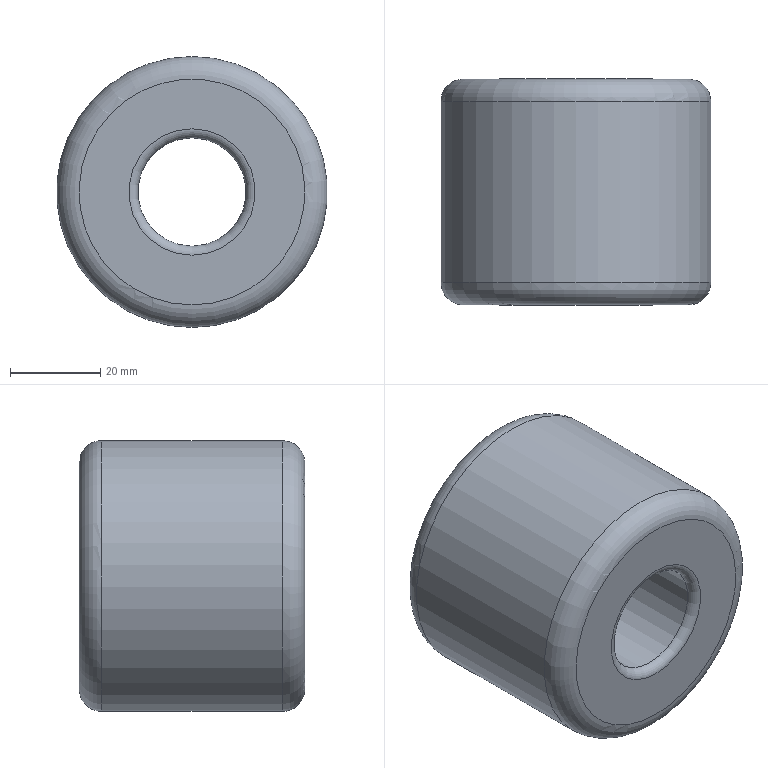Part | NX | features solid 2 | 1 solid | 8 faces | box 60 x 50 x 60 mm | volume 116671 mm3 | torus 4 | cylinder 2 | plane 2 | commonest cylinder face diameters 24 x1 60 x1
STEP:
#1=CARTESIAN_POINT('',(460.,445.,-55.));
#2=VERTEX_POINT('',#1);
#3=CARTESIAN_POINT('',(460.,445.,-25.));
#4=DIRECTION('',(0.,-1.,0.));
#5=DIRECTION('',(0.,0.,-1.));
#6=AXIS2_PLACEMENT_3D('',#3,#4,#5);
#7=CIRCLE('',#6,30.);
#8=EDGE_CURVE('',#2,#2,#7,.F.);
#9=ORIENTED_EDGE('',*,*,#8,.F.);
#10=EDGE_LOOP('',(#9));
#11=FACE_BOUND('',#10,.T.);
#12=CARTESIAN_POINT('',(460.,405.,-55.));
#13=VERTEX_POINT('',#12);
#14=CARTESIAN_POINT('',(460.,405.,-25.));
#15=DIRECTION('',(0.,-1.,0.));
#16=DIRECTION('',(0.,0.,-1.));
#17=AXIS2_PLACEMENT_3D('',#14,#15,#16);
#18=CIRCLE('',#17,30.);
#19=EDGE_CURVE('',#13,#13,#18,.T.);
#20=ORIENTED_EDGE('',*,*,#19,.F.);
#21=EDGE_LOOP('',(#20));
#22=FACE_BOUND('',#21,.T.);
#23=CARTESIAN_POINT('',(460.,400.,-25.));
#24=DIRECTION('',(0.,1.,0.));
#25=DIRECTION('',(0.,0.,-1.));
#26=AXIS2_PLACEMENT_3D('',#23,#24,#25);
#27=CYLINDRICAL_SURFACE('',#26,30.);
#28=ADVANCED_FACE('',(#11,#22),#27,.T.);
#29=CARTESIAN_POINT('',(460.,400.,-39.));
#30=VERTEX_POINT('',#29);
#31=CARTESIAN_POINT('',(460.,400.,-25.));
#32=DIRECTION('',(0.,-1.,0.));
#33=DIRECTION('',(0.,0.,-1.));
#34=AXIS2_PLACEMENT_3D('',#31,#32,#33);
#35=CIRCLE('',#34,14.);
#36=EDGE_CURVE('',#30,#30,#35,.T.);
#37=ORIENTED_EDGE('',*,*,#36,.F.);
#38=EDGE_LOOP('',(#37));
#39=FACE_BOUND('',#38,.T.);
#40=CARTESIAN_POINT('',(460.,400.,-50.));
#41=VERTEX_POINT('',#40);
#42=CARTESIAN_POINT('',(460.,400.,-25.));
#43=DIRECTION('',(0.,-1.,0.));
#44=DIRECTION('',(0.,0.,-1.));
#45=AXIS2_PLACEMENT_3D('',#42,#43,#44);
#46=CIRCLE('',#45,25.);
#47=EDGE_CURVE('',#41,#41,#46,.F.);
#48=ORIENTED_EDGE('',*,*,#47,.F.);
#49=EDGE_LOOP('',(#48));
#50=FACE_BOUND('',#49,.T.);
#51=CARTESIAN_POINT('',(460.,400.,-25.));
#52=DIRECTION('',(0.,1.,0.));
#53=DIRECTION('',(0.,0.,-1.));
#54=AXIS2_PLACEMENT_3D('',#51,#52,#53);
#55=PLANE('',#54);
#56=ADVANCED_FACE('',(#39,#50),#55,.F.);
#57=CARTESIAN_POINT('',(460.,450.,-39.));
#58=VERTEX_POINT('',#57);
#59=CARTESIAN_POINT('',(460.,450.,-25.));
#60=DIRECTION('',(0.,-1.,0.));
#61=DIRECTION('',(0.,0.,-1.));
#62=AXIS2_PLACEMENT_3D('',#59,#60,#61);
#63=CIRCLE('',#62,14.);
#64=EDGE_CURVE('',#58,#58,#63,.F.);
#65=ORIENTED_EDGE('',*,*,#64,.F.);
#66=EDGE_LOOP('',(#65));
#67=FACE_BOUND('',#66,.T.);
#68=CARTESIAN_POINT('',(460.,450.,-50.));
#69=VERTEX_POINT('',#68);
#70=CARTESIAN_POINT('',(460.,450.,-25.));
#71=DIRECTION('',(0.,-1.,0.));
#72=DIRECTION('',(0.,0.,-1.));
#73=AXIS2_PLACEMENT_3D('',#70,#71,#72);
#74=CIRCLE('',#73,25.);
#75=EDGE_CURVE('',#69,#69,#74,.T.);
#76=ORIENTED_EDGE('',*,*,#75,.F.);
#77=EDGE_LOOP('',(#76));
#78=FACE_BOUND('',#77,.T.);
#79=CARTESIAN_POINT('',(460.,450.,-25.));
#80=DIRECTION('',(0.,1.,0.));
#81=DIRECTION('',(0.,0.,-1.));
#82=AXIS2_PLACEMENT_3D('',#79,#80,#81);
#83=PLANE('',#82);
#84=ADVANCED_FACE('',(#67,#78),#83,.T.);
#85=CARTESIAN_POINT('',(460.,448.,-37.));
#86=VERTEX_POINT('',#85);
#87=CARTESIAN_POINT('',(460.,448.,-25.));
#88=DIRECTION('',(0.,-1.,0.));
#89=DIRECTION('',(0.,0.,-1.));
#90=AXIS2_PLACEMENT_3D('',#87,#88,#89);
#91=CIRCLE('',#90,12.);
#92=EDGE_CURVE('',#86,#86,#91,.T.);
#93=ORIENTED_EDGE('',*,*,#92,.F.);
#94=EDGE_LOOP('',(#93));
#95=FACE_BOUND('',#94,.T.);
#96=CARTESIAN_POINT('',(460.,402.,-37.));
#97=VERTEX_POINT('',#96);
#98=CARTESIAN_POINT('',(460.,402.,-25.));
#99=DIRECTION('',(0.,-1.,0.));
#100=DIRECTION('',(0.,0.,-1.));
#101=AXIS2_PLACEMENT_3D('',#98,#99,#100);
#102=CIRCLE('',#101,12.);
#103=EDGE_CURVE('',#97,#97,#102,.F.);
#104=ORIENTED_EDGE('',*,*,#103,.F.);
#105=EDGE_LOOP('',(#104));
#106=FACE_BOUND('',#105,.T.);
#107=CARTESIAN_POINT('',(460.,400.,-25.));
#108=DIRECTION('',(0.,1.,0.));
#109=DIRECTION('',(0.,0.,-1.));
#110=AXIS2_PLACEMENT_3D('',#107,#108,#109);
#111=CYLINDRICAL_SURFACE('',#110,12.);
#112=ADVANCED_FACE('',(#95,#106),#111,.F.);
#113=ORIENTED_EDGE('',*,*,#8,.T.);
#114=EDGE_LOOP('',(#113));
#115=FACE_BOUND('',#114,.T.);
#116=ORIENTED_EDGE('',*,*,#75,.T.);
#117=EDGE_LOOP('',(#116));
#118=FACE_BOUND('',#117,.T.);
#119=CARTESIAN_POINT('',(460.,445.,-25.));
#120=DIRECTION('',(0.,1.,0.));
#121=DIRECTION('',(0.,0.,-1.));
#122=AXIS2_PLACEMENT_3D('',#119,#120,#121);
#123=TOROIDAL_SURFACE('',#122,25.,5.);
#124=ADVANCED_FACE('',(#115,#118),#123,.T.);
#125=ORIENTED_EDGE('',*,*,#47,.T.);
#126=EDGE_LOOP('',(#125));
#127=FACE_BOUND('',#126,.T.);
#128=ORIENTED_EDGE('',*,*,#19,.T.);
#129=EDGE_LOOP('',(#128));
#130=FACE_BOUND('',#129,.T.);
#131=CARTESIAN_POINT('',(460.,405.,-25.));
#132=DIRECTION('',(0.,1.,0.));
#133=DIRECTION('',(0.,0.,-1.));
#134=AXIS2_PLACEMENT_3D('',#131,#132,#133);
#135=TOROIDAL_SURFACE('',#134,25.,5.);
#136=ADVANCED_FACE('',(#127,#130),#135,.T.);
#137=ORIENTED_EDGE('',*,*,#64,.T.);
#138=EDGE_LOOP('',(#137));
#139=FACE_BOUND('',#138,.T.);
#140=ORIENTED_EDGE('',*,*,#92,.T.);
#141=EDGE_LOOP('',(#140));
#142=FACE_BOUND('',#141,.T.);
#143=CARTESIAN_POINT('',(460.,448.,-25.));
#144=DIRECTION('',(0.,1.,0.));
#145=DIRECTION('',(0.,0.,-1.));
#146=AXIS2_PLACEMENT_3D('',#143,#144,#145);
#147=TOROIDAL_SURFACE('',#146,14.,2.);
#148=ADVANCED_FACE('',(#139,#142),#147,.T.);
#149=ORIENTED_EDGE('',*,*,#103,.T.);
#150=EDGE_LOOP('',(#149));
#151=FACE_BOUND('',#150,.T.);
#152=ORIENTED_EDGE('',*,*,#36,.T.);
#153=EDGE_LOOP('',(#152));
#154=FACE_BOUND('',#153,.T.);
#155=CARTESIAN_POINT('',(460.,402.,-25.));
#156=DIRECTION('',(0.,1.,0.));
#157=DIRECTION('',(0.,0.,-1.));
#158=AXIS2_PLACEMENT_3D('',#155,#156,#157);
#159=TOROIDAL_SURFACE('',#158,14.,2.);
#160=ADVANCED_FACE('',(#151,#154),#159,.T.);
#161=CLOSED_SHELL('',(#28,#56,#84,#112,#124,#136,#148,#160));
#162=MANIFOLD_SOLID_BREP('',#161);
#163=(LENGTH_UNIT()NAMED_UNIT(*)SI_UNIT(.MILLI.,.METRE.));
#164=UNCERTAINTY_MEASURE_WITH_UNIT(LENGTH_MEASURE(0.00001),#163,'','');
#165=(NAMED_UNIT(*)PLANE_ANGLE_UNIT()SI_UNIT($,.RADIAN.));
#166=(NAMED_UNIT(*)SI_UNIT($,.STERADIAN.)SOLID_ANGLE_UNIT());
#167=(GEOMETRIC_REPRESENTATION_CONTEXT(3)GLOBAL_UNCERTAINTY_ASSIGNED_CONTEXT((#164))GLOBAL_UNIT_ASSIGNED_CONTEXT((#163,#165,#166))REPRESENTATION_CONTEXT('',''));
#168=ADVANCED_BREP_SHAPE_REPRESENTATION('',(#162),#167);